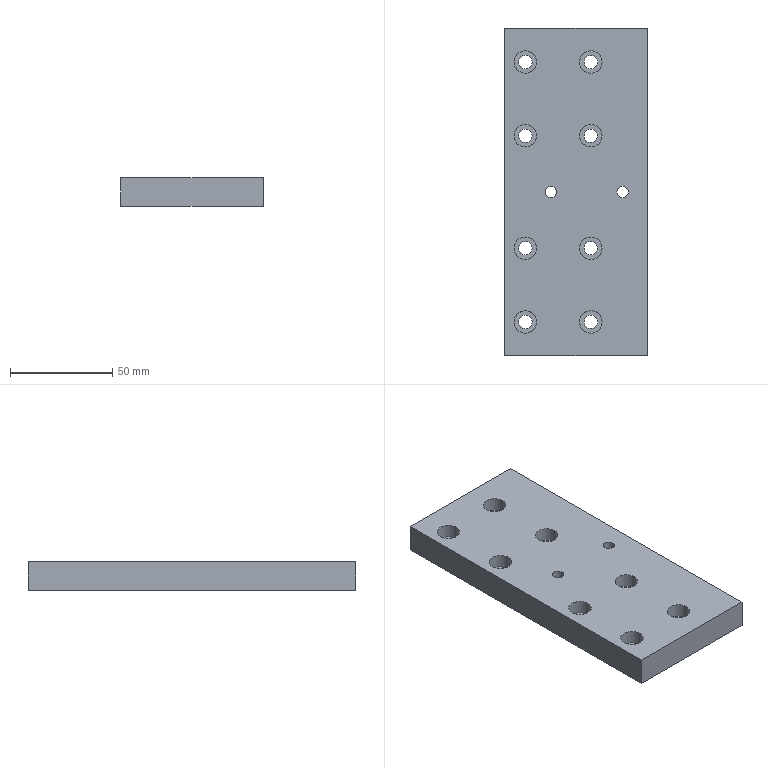Part | NX | 1 solid | 40 faces | box 69.5 x 160 x 14 mm | volume 146674 mm3 | cylinder 22 | plane 16 | cone 2 | commonest cylinder face diameters 6.6 x8 11 x8 5 x2 5.5 x2 10 x2
STEP:
#1=CARTESIAN_POINT('',(-34.75,80.,-7.));
#2=VERTEX_POINT('',#1);
#3=CARTESIAN_POINT('',(-34.75,-80.,-7.));
#4=VERTEX_POINT('',#3);
#5=CARTESIAN_POINT('',(-34.75,80.,-7.));
#6=DIRECTION('',(0.,-1.,0.));
#7=VECTOR('',#6,1000.);
#8=LINE('',#5,#7);
#9=EDGE_CURVE('',#2,#4,#8,.T.);
#10=ORIENTED_EDGE('',*,*,#9,.T.);
#11=CARTESIAN_POINT('',(-34.75,-80.,7.));
#12=VERTEX_POINT('',#11);
#13=CARTESIAN_POINT('',(-34.75,-80.,7.));
#14=DIRECTION('',(0.,0.,-1.));
#15=VECTOR('',#14,1000.);
#16=LINE('',#13,#15);
#17=EDGE_CURVE('',#12,#4,#16,.T.);
#18=ORIENTED_EDGE('',*,*,#17,.F.);
#19=CARTESIAN_POINT('',(-34.75,80.,7.));
#20=VERTEX_POINT('',#19);
#21=CARTESIAN_POINT('',(-34.75,80.,7.));
#22=DIRECTION('',(0.,-1.,0.));
#23=VECTOR('',#22,1000.);
#24=LINE('',#21,#23);
#25=EDGE_CURVE('',#20,#12,#24,.T.);
#26=ORIENTED_EDGE('',*,*,#25,.F.);
#27=CARTESIAN_POINT('',(-34.75,80.,7.));
#28=DIRECTION('',(0.,0.,-1.));
#29=VECTOR('',#28,1000.);
#30=LINE('',#27,#29);
#31=EDGE_CURVE('',#20,#2,#30,.T.);
#32=ORIENTED_EDGE('',*,*,#31,.T.);
#33=EDGE_LOOP('',(#10,#18,#26,#32));
#34=FACE_BOUND('',#33,.T.);
#35=CARTESIAN_POINT('',(-34.75,80.,7.));
#36=DIRECTION('',(1.,0.,0.));
#37=DIRECTION('',(0.,1.,0.));
#38=AXIS2_PLACEMENT_3D('',#35,#36,#37);
#39=PLANE('',#38);
#40=ADVANCED_FACE('',(#34),#39,.F.);
#41=CARTESIAN_POINT('',(34.75,-80.,-7.));
#42=VERTEX_POINT('',#41);
#43=CARTESIAN_POINT('',(34.75,-80.,-7.));
#44=DIRECTION('',(1.,0.,0.));
#45=VECTOR('',#44,1000.);
#46=LINE('',#43,#45);
#47=EDGE_CURVE('',#4,#42,#46,.T.);
#48=ORIENTED_EDGE('',*,*,#47,.T.);
#49=CARTESIAN_POINT('',(34.75,-80.,7.));
#50=VERTEX_POINT('',#49);
#51=CARTESIAN_POINT('',(34.75,-80.,7.));
#52=DIRECTION('',(0.,0.,-1.));
#53=VECTOR('',#52,1000.);
#54=LINE('',#51,#53);
#55=EDGE_CURVE('',#50,#42,#54,.T.);
#56=ORIENTED_EDGE('',*,*,#55,.F.);
#57=CARTESIAN_POINT('',(34.75,-80.,7.));
#58=DIRECTION('',(1.,0.,0.));
#59=VECTOR('',#58,1000.);
#60=LINE('',#57,#59);
#61=EDGE_CURVE('',#12,#50,#60,.T.);
#62=ORIENTED_EDGE('',*,*,#61,.F.);
#63=ORIENTED_EDGE('',*,*,#17,.T.);
#64=EDGE_LOOP('',(#48,#56,#62,#63));
#65=FACE_BOUND('',#64,.T.);
#66=CARTESIAN_POINT('',(34.75,-80.,7.));
#67=DIRECTION('',(0.,1.,0.));
#68=DIRECTION('',(0.,0.,1.));
#69=AXIS2_PLACEMENT_3D('',#66,#67,#68);
#70=PLANE('',#69);
#71=ADVANCED_FACE('',(#65),#70,.F.);
#72=CARTESIAN_POINT('',(34.75,32.5,-3.));
#73=VERTEX_POINT('',#72);
#74=CARTESIAN_POINT('',(34.75,32.5,-0.5));
#75=DIRECTION('',(1.,0.,0.));
#76=DIRECTION('',(0.,0.,-1.));
#77=AXIS2_PLACEMENT_3D('',#74,#75,#76);
#78=CIRCLE('',#77,2.5);
#79=EDGE_CURVE('',#73,#73,#78,.T.);
#80=ORIENTED_EDGE('',*,*,#79,.F.);
#81=EDGE_LOOP('',(#80));
#82=FACE_BOUND('',#81,.T.);
#83=CARTESIAN_POINT('',(34.75,-32.5,-3.));
#84=VERTEX_POINT('',#83);
#85=CARTESIAN_POINT('',(34.75,-32.5,-0.5));
#86=DIRECTION('',(1.,0.,0.));
#87=DIRECTION('',(0.,0.,-1.));
#88=AXIS2_PLACEMENT_3D('',#85,#86,#87);
#89=CIRCLE('',#88,2.5);
#90=EDGE_CURVE('',#84,#84,#89,.T.);
#91=ORIENTED_EDGE('',*,*,#90,.F.);
#92=EDGE_LOOP('',(#91));
#93=FACE_BOUND('',#92,.T.);
#94=CARTESIAN_POINT('',(34.75,80.,-7.));
#95=VERTEX_POINT('',#94);
#96=CARTESIAN_POINT('',(34.75,80.,-7.));
#97=DIRECTION('',(0.,1.,0.));
#98=VECTOR('',#97,1000.);
#99=LINE('',#96,#98);
#100=EDGE_CURVE('',#42,#95,#99,.T.);
#101=ORIENTED_EDGE('',*,*,#100,.T.);
#102=CARTESIAN_POINT('',(34.75,80.,7.));
#103=VERTEX_POINT('',#102);
#104=CARTESIAN_POINT('',(34.75,80.,7.));
#105=DIRECTION('',(0.,0.,-1.));
#106=VECTOR('',#105,1000.);
#107=LINE('',#104,#106);
#108=EDGE_CURVE('',#103,#95,#107,.T.);
#109=ORIENTED_EDGE('',*,*,#108,.F.);
#110=CARTESIAN_POINT('',(34.75,80.,7.));
#111=DIRECTION('',(0.,1.,0.));
#112=VECTOR('',#111,1000.);
#113=LINE('',#110,#112);
#114=EDGE_CURVE('',#50,#103,#113,.T.);
#115=ORIENTED_EDGE('',*,*,#114,.F.);
#116=ORIENTED_EDGE('',*,*,#55,.T.);
#117=EDGE_LOOP('',(#101,#109,#115,#116));
#118=FACE_BOUND('',#117,.T.);
#119=CARTESIAN_POINT('',(34.75,80.,7.));
#120=DIRECTION('',(-1.,0.,0.));
#121=DIRECTION('',(0.,-1.,0.));
#122=AXIS2_PLACEMENT_3D('',#119,#120,#121);
#123=PLANE('',#122);
#124=ADVANCED_FACE('',(#82,#93,#118),#123,.F.);
#125=CARTESIAN_POINT('',(34.75,80.,-7.));
#126=DIRECTION('',(-1.,0.,0.));
#127=VECTOR('',#126,1000.);
#128=LINE('',#125,#127);
#129=EDGE_CURVE('',#95,#2,#128,.T.);
#130=ORIENTED_EDGE('',*,*,#129,.T.);
#131=ORIENTED_EDGE('',*,*,#31,.F.);
#132=CARTESIAN_POINT('',(34.75,80.,7.));
#133=DIRECTION('',(-1.,0.,0.));
#134=VECTOR('',#133,1000.);
#135=LINE('',#132,#134);
#136=EDGE_CURVE('',#103,#20,#135,.T.);
#137=ORIENTED_EDGE('',*,*,#136,.F.);
#138=ORIENTED_EDGE('',*,*,#108,.T.);
#139=EDGE_LOOP('',(#130,#131,#137,#138));
#140=FACE_BOUND('',#139,.T.);
#141=CARTESIAN_POINT('',(34.75,80.,7.));
#142=DIRECTION('',(0.,-1.,0.));
#143=DIRECTION('',(0.,0.,-1.));
#144=AXIS2_PLACEMENT_3D('',#141,#142,#143);
#145=PLANE('',#144);
#146=ADVANCED_FACE('',(#140),#145,.F.);
#147=CARTESIAN_POINT('',(-15.,0.,7.));
#148=VERTEX_POINT('',#147);
#149=CARTESIAN_POINT('',(-12.25,0.,7.));
#150=DIRECTION('',(0.,0.,-1.));
#151=DIRECTION('',(-1.,0.,0.));
#152=AXIS2_PLACEMENT_3D('',#149,#150,#151);
#153=CIRCLE('',#152,2.75);
#154=EDGE_CURVE('',#148,#148,#153,.T.);
#155=ORIENTED_EDGE('',*,*,#154,.T.);
#156=EDGE_LOOP('',(#155));
#157=FACE_BOUND('',#156,.T.);
#158=CARTESIAN_POINT('',(20.,0.,7.));
#159=VERTEX_POINT('',#158);
#160=CARTESIAN_POINT('',(22.75,0.,7.));
#161=DIRECTION('',(0.,0.,-1.));
#162=DIRECTION('',(-1.,0.,0.));
#163=AXIS2_PLACEMENT_3D('',#160,#161,#162);
#164=CIRCLE('',#163,2.75);
#165=EDGE_CURVE('',#159,#159,#164,.T.);
#166=ORIENTED_EDGE('',*,*,#165,.T.);
#167=EDGE_LOOP('',(#166));
#168=FACE_BOUND('',#167,.T.);
#169=CARTESIAN_POINT('',(-19.25,27.5,7.));
#170=VERTEX_POINT('',#169);
#171=CARTESIAN_POINT('',(-24.75,27.5,7.));
#172=DIRECTION('',(0.,0.,1.));
#173=DIRECTION('',(1.,0.,0.));
#174=AXIS2_PLACEMENT_3D('',#171,#172,#173);
#175=CIRCLE('',#174,5.5);
#176=EDGE_CURVE('',#170,#170,#175,.T.);
#177=ORIENTED_EDGE('',*,*,#176,.F.);
#178=EDGE_LOOP('',(#177));
#179=FACE_BOUND('',#178,.T.);
#180=CARTESIAN_POINT('',(12.75,27.5,7.));
#181=VERTEX_POINT('',#180);
#182=CARTESIAN_POINT('',(7.25,27.5,7.));
#183=DIRECTION('',(0.,0.,1.));
#184=DIRECTION('',(1.,0.,0.));
#185=AXIS2_PLACEMENT_3D('',#182,#183,#184);
#186=CIRCLE('',#185,5.5);
#187=EDGE_CURVE('',#181,#181,#186,.T.);
#188=ORIENTED_EDGE('',*,*,#187,.F.);
#189=EDGE_LOOP('',(#188));
#190=FACE_BOUND('',#189,.T.);
#191=CARTESIAN_POINT('',(12.75,-27.5,7.));
#192=VERTEX_POINT('',#191);
#193=CARTESIAN_POINT('',(7.25,-27.5,7.));
#194=DIRECTION('',(0.,0.,1.));
#195=DIRECTION('',(1.,0.,0.));
#196=AXIS2_PLACEMENT_3D('',#193,#194,#195);
#197=CIRCLE('',#196,5.5);
#198=EDGE_CURVE('',#192,#192,#197,.T.);
#199=ORIENTED_EDGE('',*,*,#198,.F.);
#200=EDGE_LOOP('',(#199));
#201=FACE_BOUND('',#200,.T.);
#202=CARTESIAN_POINT('',(-19.25,-27.5,7.));
#203=VERTEX_POINT('',#202);
#204=CARTESIAN_POINT('',(-24.75,-27.5,7.));
#205=DIRECTION('',(0.,0.,1.));
#206=DIRECTION('',(1.,0.,0.));
#207=AXIS2_PLACEMENT_3D('',#204,#205,#206);
#208=CIRCLE('',#207,5.5);
#209=EDGE_CURVE('',#203,#203,#208,.T.);
#210=ORIENTED_EDGE('',*,*,#209,.F.);
#211=EDGE_LOOP('',(#210));
#212=FACE_BOUND('',#211,.T.);
#213=CARTESIAN_POINT('',(12.75,63.5,7.));
#214=VERTEX_POINT('',#213);
#215=CARTESIAN_POINT('',(7.25,63.5,7.));
#216=DIRECTION('',(0.,0.,1.));
#217=DIRECTION('',(1.,0.,0.));
#218=AXIS2_PLACEMENT_3D('',#215,#216,#217);
#219=CIRCLE('',#218,5.5);
#220=EDGE_CURVE('',#214,#214,#219,.T.);
#221=ORIENTED_EDGE('',*,*,#220,.F.);
#222=EDGE_LOOP('',(#221));
#223=FACE_BOUND('',#222,.T.);
#224=CARTESIAN_POINT('',(-19.25,63.5,7.));
#225=VERTEX_POINT('',#224);
#226=CARTESIAN_POINT('',(-24.75,63.5,7.));
#227=DIRECTION('',(0.,0.,1.));
#228=DIRECTION('',(1.,0.,0.));
#229=AXIS2_PLACEMENT_3D('',#226,#227,#228);
#230=CIRCLE('',#229,5.5);
#231=EDGE_CURVE('',#225,#225,#230,.T.);
#232=ORIENTED_EDGE('',*,*,#231,.F.);
#233=EDGE_LOOP('',(#232));
#234=FACE_BOUND('',#233,.T.);
#235=CARTESIAN_POINT('',(-19.25,-63.5,7.));
#236=VERTEX_POINT('',#235);
#237=CARTESIAN_POINT('',(-24.75,-63.5,7.));
#238=DIRECTION('',(0.,0.,1.));
#239=DIRECTION('',(1.,0.,0.));
#240=AXIS2_PLACEMENT_3D('',#237,#238,#239);
#241=CIRCLE('',#240,5.5);
#242=EDGE_CURVE('',#236,#236,#241,.T.);
#243=ORIENTED_EDGE('',*,*,#242,.F.);
#244=EDGE_LOOP('',(#243));
#245=FACE_BOUND('',#244,.T.);
#246=CARTESIAN_POINT('',(12.75,-63.5,7.));
#247=VERTEX_POINT('',#246);
#248=CARTESIAN_POINT('',(7.25,-63.5,7.));
#249=DIRECTION('',(0.,0.,1.));
#250=DIRECTION('',(1.,0.,0.));
#251=AXIS2_PLACEMENT_3D('',#248,#249,#250);
#252=CIRCLE('',#251,5.5);
#253=EDGE_CURVE('',#247,#247,#252,.T.);
#254=ORIENTED_EDGE('',*,*,#253,.F.);
#255=EDGE_LOOP('',(#254));
#256=FACE_BOUND('',#255,.T.);
#257=ORIENTED_EDGE('',*,*,#25,.T.);
#258=ORIENTED_EDGE('',*,*,#61,.T.);
#259=ORIENTED_EDGE('',*,*,#114,.T.);
#260=ORIENTED_EDGE('',*,*,#136,.T.);
#261=EDGE_LOOP('',(#257,#258,#259,#260));
#262=FACE_BOUND('',#261,.T.);
#263=CARTESIAN_POINT('',(0.,0.,7.));
#264=DIRECTION('',(0.,0.,-1.));
#265=DIRECTION('',(-1.,0.,0.));
#266=AXIS2_PLACEMENT_3D('',#263,#264,#265);
#267=PLANE('',#266);
#268=ADVANCED_FACE('',(#157,#168,#179,#190,#201,#212,#223,#234,#245,#256,#262),#267,.F.);
#269=CARTESIAN_POINT('',(-17.25,0.,-7.));
#270=VERTEX_POINT('',#269);
#271=CARTESIAN_POINT('',(-12.25,0.,-7.));
#272=DIRECTION('',(0.,0.,-1.));
#273=DIRECTION('',(-1.,0.,0.));
#274=AXIS2_PLACEMENT_3D('',#271,#272,#273);
#275=CIRCLE('',#274,5.);
#276=EDGE_CURVE('',#270,#270,#275,.T.);
#277=ORIENTED_EDGE('',*,*,#276,.F.);
#278=EDGE_LOOP('',(#277));
#279=FACE_BOUND('',#278,.T.);
#280=CARTESIAN_POINT('',(17.75,0.,-7.));
#281=VERTEX_POINT('',#280);
#282=CARTESIAN_POINT('',(22.75,0.,-7.));
#283=DIRECTION('',(0.,0.,-1.));
#284=DIRECTION('',(-1.,0.,0.));
#285=AXIS2_PLACEMENT_3D('',#282,#283,#284);
#286=CIRCLE('',#285,5.);
#287=EDGE_CURVE('',#281,#281,#286,.T.);
#288=ORIENTED_EDGE('',*,*,#287,.F.);
#289=EDGE_LOOP('',(#288));
#290=FACE_BOUND('',#289,.T.);
#291=CARTESIAN_POINT('',(-21.45,27.5,-7.));
#292=VERTEX_POINT('',#291);
#293=CARTESIAN_POINT('',(-24.75,27.5,-7.));
#294=DIRECTION('',(0.,0.,1.));
#295=DIRECTION('',(1.,0.,0.));
#296=AXIS2_PLACEMENT_3D('',#293,#294,#295);
#297=CIRCLE('',#296,3.3);
#298=EDGE_CURVE('',#292,#292,#297,.T.);
#299=ORIENTED_EDGE('',*,*,#298,.T.);
#300=EDGE_LOOP('',(#299));
#301=FACE_BOUND('',#300,.T.);
#302=CARTESIAN_POINT('',(10.55,27.5,-7.));
#303=VERTEX_POINT('',#302);
#304=CARTESIAN_POINT('',(7.25,27.5,-7.));
#305=DIRECTION('',(0.,0.,1.));
#306=DIRECTION('',(1.,0.,0.));
#307=AXIS2_PLACEMENT_3D('',#304,#305,#306);
#308=CIRCLE('',#307,3.3);
#309=EDGE_CURVE('',#303,#303,#308,.T.);
#310=ORIENTED_EDGE('',*,*,#309,.T.);
#311=EDGE_LOOP('',(#310));
#312=FACE_BOUND('',#311,.T.);
#313=CARTESIAN_POINT('',(10.55,-27.5,-7.));
#314=VERTEX_POINT('',#313);
#315=CARTESIAN_POINT('',(7.25,-27.5,-7.));
#316=DIRECTION('',(0.,0.,1.));
#317=DIRECTION('',(1.,0.,0.));
#318=AXIS2_PLACEMENT_3D('',#315,#316,#317);
#319=CIRCLE('',#318,3.3);
#320=EDGE_CURVE('',#314,#314,#319,.T.);
#321=ORIENTED_EDGE('',*,*,#320,.T.);
#322=EDGE_LOOP('',(#321));
#323=FACE_BOUND('',#322,.T.);
#324=CARTESIAN_POINT('',(-21.45,-27.5,-7.));
#325=VERTEX_POINT('',#324);
#326=CARTESIAN_POINT('',(-24.75,-27.5,-7.));
#327=DIRECTION('',(0.,0.,1.));
#328=DIRECTION('',(1.,0.,0.));
#329=AXIS2_PLACEMENT_3D('',#326,#327,#328);
#330=CIRCLE('',#329,3.3);
#331=EDGE_CURVE('',#325,#325,#330,.T.);
#332=ORIENTED_EDGE('',*,*,#331,.T.);
#333=EDGE_LOOP('',(#332));
#334=FACE_BOUND('',#333,.T.);
#335=CARTESIAN_POINT('',(10.55,63.5,-7.));
#336=VERTEX_POINT('',#335);
#337=CARTESIAN_POINT('',(7.25,63.5,-7.));
#338=DIRECTION('',(0.,0.,1.));
#339=DIRECTION('',(1.,0.,0.));
#340=AXIS2_PLACEMENT_3D('',#337,#338,#339);
#341=CIRCLE('',#340,3.3);
#342=EDGE_CURVE('',#336,#336,#341,.T.);
#343=ORIENTED_EDGE('',*,*,#342,.T.);
#344=EDGE_LOOP('',(#343));
#345=FACE_BOUND('',#344,.T.);
#346=CARTESIAN_POINT('',(-21.45,63.5,-7.));
#347=VERTEX_POINT('',#346);
#348=CARTESIAN_POINT('',(-24.75,63.5,-7.));
#349=DIRECTION('',(0.,0.,1.));
#350=DIRECTION('',(1.,0.,0.));
#351=AXIS2_PLACEMENT_3D('',#348,#349,#350);
#352=CIRCLE('',#351,3.3);
#353=EDGE_CURVE('',#347,#347,#352,.T.);
#354=ORIENTED_EDGE('',*,*,#353,.T.);
#355=EDGE_LOOP('',(#354));
#356=FACE_BOUND('',#355,.T.);
#357=CARTESIAN_POINT('',(-21.45,-63.5,-7.));
#358=VERTEX_POINT('',#357);
#359=CARTESIAN_POINT('',(-24.75,-63.5,-7.));
#360=DIRECTION('',(0.,0.,1.));
#361=DIRECTION('',(1.,0.,0.));
#362=AXIS2_PLACEMENT_3D('',#359,#360,#361);
#363=CIRCLE('',#362,3.3);
#364=EDGE_CURVE('',#358,#358,#363,.T.);
#365=ORIENTED_EDGE('',*,*,#364,.T.);
#366=EDGE_LOOP('',(#365));
#367=FACE_BOUND('',#366,.T.);
#368=CARTESIAN_POINT('',(10.55,-63.5,-7.));
#369=VERTEX_POINT('',#368);
#370=CARTESIAN_POINT('',(7.25,-63.5,-7.));
#371=DIRECTION('',(0.,0.,1.));
#372=DIRECTION('',(1.,0.,0.));
#373=AXIS2_PLACEMENT_3D('',#370,#371,#372);
#374=CIRCLE('',#373,3.3);
#375=EDGE_CURVE('',#369,#369,#374,.T.);
#376=ORIENTED_EDGE('',*,*,#375,.T.);
#377=EDGE_LOOP('',(#376));
#378=FACE_BOUND('',#377,.T.);
#379=ORIENTED_EDGE('',*,*,#9,.F.);
#380=ORIENTED_EDGE('',*,*,#129,.F.);
#381=ORIENTED_EDGE('',*,*,#100,.F.);
#382=ORIENTED_EDGE('',*,*,#47,.F.);
#383=EDGE_LOOP('',(#379,#380,#381,#382));
#384=FACE_BOUND('',#383,.T.);
#385=CARTESIAN_POINT('',(0.,0.,-7.));
#386=DIRECTION('',(0.,0.,-1.));
#387=DIRECTION('',(-1.,0.,0.));
#388=AXIS2_PLACEMENT_3D('',#385,#386,#387);
#389=PLANE('',#388);
#390=ADVANCED_FACE('',(#279,#290,#301,#312,#323,#334,#345,#356,#367,#378,#384),#389,.T.);
#391=ORIENTED_EDGE('',*,*,#375,.F.);
#392=EDGE_LOOP('',(#391));
#393=FACE_BOUND('',#392,.T.);
#394=CARTESIAN_POINT('',(10.55,-63.5,0.2));
#395=VERTEX_POINT('',#394);
#396=CARTESIAN_POINT('',(7.25,-63.5,0.2));
#397=DIRECTION('',(0.,0.,1.));
#398=DIRECTION('',(1.,0.,0.));
#399=AXIS2_PLACEMENT_3D('',#396,#397,#398);
#400=CIRCLE('',#399,3.3);
#401=EDGE_CURVE('',#395,#395,#400,.T.);
#402=ORIENTED_EDGE('',*,*,#401,.T.);
#403=EDGE_LOOP('',(#402));
#404=FACE_BOUND('',#403,.T.);
#405=CARTESIAN_POINT('',(7.25,-63.5,7.));
#406=DIRECTION('',(0.,0.,1.));
#407=DIRECTION('',(1.,0.,0.));
#408=AXIS2_PLACEMENT_3D('',#405,#406,#407);
#409=CYLINDRICAL_SURFACE('',#408,3.3);
#410=ADVANCED_FACE('',(#393,#404),#409,.F.);
#411=ORIENTED_EDGE('',*,*,#401,.F.);
#412=EDGE_LOOP('',(#411));
#413=FACE_BOUND('',#412,.T.);
#414=CARTESIAN_POINT('',(12.75,-63.5,0.2));
#415=VERTEX_POINT('',#414);
#416=CARTESIAN_POINT('',(7.25,-63.5,0.2));
#417=DIRECTION('',(0.,0.,1.));
#418=DIRECTION('',(1.,0.,0.));
#419=AXIS2_PLACEMENT_3D('',#416,#417,#418);
#420=CIRCLE('',#419,5.5);
#421=EDGE_CURVE('',#415,#415,#420,.T.);
#422=ORIENTED_EDGE('',*,*,#421,.T.);
#423=EDGE_LOOP('',(#422));
#424=FACE_BOUND('',#423,.T.);
#425=CARTESIAN_POINT('',(10.55,-63.5,0.2));
#426=DIRECTION('',(0.,0.,-1.));
#427=DIRECTION('',(-1.,0.,0.));
#428=AXIS2_PLACEMENT_3D('',#425,#426,#427);
#429=PLANE('',#428);
#430=ADVANCED_FACE('',(#413,#424),#429,.F.);
#431=ORIENTED_EDGE('',*,*,#421,.F.);
#432=EDGE_LOOP('',(#431));
#433=FACE_BOUND('',#432,.T.);
#434=ORIENTED_EDGE('',*,*,#253,.T.);
#435=EDGE_LOOP('',(#434));
#436=FACE_BOUND('',#435,.T.);
#437=CARTESIAN_POINT('',(7.25,-63.5,7.));
#438=DIRECTION('',(0.,0.,1.));
#439=DIRECTION('',(1.,0.,0.));
#440=AXIS2_PLACEMENT_3D('',#437,#438,#439);
#441=CYLINDRICAL_SURFACE('',#440,5.5);
#442=ADVANCED_FACE('',(#433,#436),#441,.F.);
#443=ORIENTED_EDGE('',*,*,#364,.F.);
#444=EDGE_LOOP('',(#443));
#445=FACE_BOUND('',#444,.T.);
#446=CARTESIAN_POINT('',(-21.45,-63.5,0.2));
#447=VERTEX_POINT('',#446);
#448=CARTESIAN_POINT('',(-24.75,-63.5,0.2));
#449=DIRECTION('',(0.,0.,1.));
#450=DIRECTION('',(1.,0.,0.));
#451=AXIS2_PLACEMENT_3D('',#448,#449,#450);
#452=CIRCLE('',#451,3.3);
#453=EDGE_CURVE('',#447,#447,#452,.T.);
#454=ORIENTED_EDGE('',*,*,#453,.T.);
#455=EDGE_LOOP('',(#454));
#456=FACE_BOUND('',#455,.T.);
#457=CARTESIAN_POINT('',(-24.75,-63.5,7.));
#458=DIRECTION('',(0.,0.,1.));
#459=DIRECTION('',(1.,0.,0.));
#460=AXIS2_PLACEMENT_3D('',#457,#458,#459);
#461=CYLINDRICAL_SURFACE('',#460,3.3);
#462=ADVANCED_FACE('',(#445,#456),#461,.F.);
#463=ORIENTED_EDGE('',*,*,#453,.F.);
#464=EDGE_LOOP('',(#463));
#465=FACE_BOUND('',#464,.T.);
#466=CARTESIAN_POINT('',(-19.25,-63.5,0.2));
#467=VERTEX_POINT('',#466);
#468=CARTESIAN_POINT('',(-24.75,-63.5,0.2));
#469=DIRECTION('',(0.,0.,1.));
#470=DIRECTION('',(1.,0.,0.));
#471=AXIS2_PLACEMENT_3D('',#468,#469,#470);
#472=CIRCLE('',#471,5.5);
#473=EDGE_CURVE('',#467,#467,#472,.T.);
#474=ORIENTED_EDGE('',*,*,#473,.T.);
#475=EDGE_LOOP('',(#474));
#476=FACE_BOUND('',#475,.T.);
#477=CARTESIAN_POINT('',(-21.45,-63.5,0.2));
#478=DIRECTION('',(0.,0.,-1.));
#479=DIRECTION('',(-1.,0.,0.));
#480=AXIS2_PLACEMENT_3D('',#477,#478,#479);
#481=PLANE('',#480);
#482=ADVANCED_FACE('',(#465,#476),#481,.F.);
#483=ORIENTED_EDGE('',*,*,#473,.F.);
#484=EDGE_LOOP('',(#483));
#485=FACE_BOUND('',#484,.T.);
#486=ORIENTED_EDGE('',*,*,#242,.T.);
#487=EDGE_LOOP('',(#486));
#488=FACE_BOUND('',#487,.T.);
#489=CARTESIAN_POINT('',(-24.75,-63.5,7.));
#490=DIRECTION('',(0.,0.,1.));
#491=DIRECTION('',(1.,0.,0.));
#492=AXIS2_PLACEMENT_3D('',#489,#490,#491);
#493=CYLINDRICAL_SURFACE('',#492,5.5);
#494=ADVANCED_FACE('',(#485,#488),#493,.F.);
#495=ORIENTED_EDGE('',*,*,#353,.F.);
#496=EDGE_LOOP('',(#495));
#497=FACE_BOUND('',#496,.T.);
#498=CARTESIAN_POINT('',(-21.45,63.5,0.2));
#499=VERTEX_POINT('',#498);
#500=CARTESIAN_POINT('',(-24.75,63.5,0.2));
#501=DIRECTION('',(0.,0.,1.));
#502=DIRECTION('',(1.,0.,0.));
#503=AXIS2_PLACEMENT_3D('',#500,#501,#502);
#504=CIRCLE('',#503,3.3);
#505=EDGE_CURVE('',#499,#499,#504,.T.);
#506=ORIENTED_EDGE('',*,*,#505,.T.);
#507=EDGE_LOOP('',(#506));
#508=FACE_BOUND('',#507,.T.);
#509=CARTESIAN_POINT('',(-24.75,63.5,7.));
#510=DIRECTION('',(0.,0.,1.));
#511=DIRECTION('',(1.,0.,0.));
#512=AXIS2_PLACEMENT_3D('',#509,#510,#511);
#513=CYLINDRICAL_SURFACE('',#512,3.3);
#514=ADVANCED_FACE('',(#497,#508),#513,.F.);
#515=ORIENTED_EDGE('',*,*,#505,.F.);
#516=EDGE_LOOP('',(#515));
#517=FACE_BOUND('',#516,.T.);
#518=CARTESIAN_POINT('',(-19.25,63.5,0.2));
#519=VERTEX_POINT('',#518);
#520=CARTESIAN_POINT('',(-24.75,63.5,0.2));
#521=DIRECTION('',(0.,0.,1.));
#522=DIRECTION('',(1.,0.,0.));
#523=AXIS2_PLACEMENT_3D('',#520,#521,#522);
#524=CIRCLE('',#523,5.5);
#525=EDGE_CURVE('',#519,#519,#524,.T.);
#526=ORIENTED_EDGE('',*,*,#525,.T.);
#527=EDGE_LOOP('',(#526));
#528=FACE_BOUND('',#527,.T.);
#529=CARTESIAN_POINT('',(-21.45,63.5,0.2));
#530=DIRECTION('',(0.,0.,-1.));
#531=DIRECTION('',(-1.,0.,0.));
#532=AXIS2_PLACEMENT_3D('',#529,#530,#531);
#533=PLANE('',#532);
#534=ADVANCED_FACE('',(#517,#528),#533,.F.);
#535=ORIENTED_EDGE('',*,*,#525,.F.);
#536=EDGE_LOOP('',(#535));
#537=FACE_BOUND('',#536,.T.);
#538=ORIENTED_EDGE('',*,*,#231,.T.);
#539=EDGE_LOOP('',(#538));
#540=FACE_BOUND('',#539,.T.);
#541=CARTESIAN_POINT('',(-24.75,63.5,7.));
#542=DIRECTION('',(0.,0.,1.));
#543=DIRECTION('',(1.,0.,0.));
#544=AXIS2_PLACEMENT_3D('',#541,#542,#543);
#545=CYLINDRICAL_SURFACE('',#544,5.5);
#546=ADVANCED_FACE('',(#537,#540),#545,.F.);
#547=ORIENTED_EDGE('',*,*,#342,.F.);
#548=EDGE_LOOP('',(#547));
#549=FACE_BOUND('',#548,.T.);
#550=CARTESIAN_POINT('',(10.55,63.5,0.2));
#551=VERTEX_POINT('',#550);
#552=CARTESIAN_POINT('',(7.25,63.5,0.2));
#553=DIRECTION('',(0.,0.,1.));
#554=DIRECTION('',(1.,0.,0.));
#555=AXIS2_PLACEMENT_3D('',#552,#553,#554);
#556=CIRCLE('',#555,3.3);
#557=EDGE_CURVE('',#551,#551,#556,.T.);
#558=ORIENTED_EDGE('',*,*,#557,.T.);
#559=EDGE_LOOP('',(#558));
#560=FACE_BOUND('',#559,.T.);
#561=CARTESIAN_POINT('',(7.25,63.5,7.));
#562=DIRECTION('',(0.,0.,1.));
#563=DIRECTION('',(1.,0.,0.));
#564=AXIS2_PLACEMENT_3D('',#561,#562,#563);
#565=CYLINDRICAL_SURFACE('',#564,3.3);
#566=ADVANCED_FACE('',(#549,#560),#565,.F.);
#567=ORIENTED_EDGE('',*,*,#557,.F.);
#568=EDGE_LOOP('',(#567));
#569=FACE_BOUND('',#568,.T.);
#570=CARTESIAN_POINT('',(12.75,63.5,0.2));
#571=VERTEX_POINT('',#570);
#572=CARTESIAN_POINT('',(7.25,63.5,0.2));
#573=DIRECTION('',(0.,0.,1.));
#574=DIRECTION('',(1.,0.,0.));
#575=AXIS2_PLACEMENT_3D('',#572,#573,#574);
#576=CIRCLE('',#575,5.5);
#577=EDGE_CURVE('',#571,#571,#576,.T.);
#578=ORIENTED_EDGE('',*,*,#577,.T.);
#579=EDGE_LOOP('',(#578));
#580=FACE_BOUND('',#579,.T.);
#581=CARTESIAN_POINT('',(10.55,63.5,0.2));
#582=DIRECTION('',(0.,0.,-1.));
#583=DIRECTION('',(-1.,0.,0.));
#584=AXIS2_PLACEMENT_3D('',#581,#582,#583);
#585=PLANE('',#584);
#586=ADVANCED_FACE('',(#569,#580),#585,.F.);
#587=ORIENTED_EDGE('',*,*,#577,.F.);
#588=EDGE_LOOP('',(#587));
#589=FACE_BOUND('',#588,.T.);
#590=ORIENTED_EDGE('',*,*,#220,.T.);
#591=EDGE_LOOP('',(#590));
#592=FACE_BOUND('',#591,.T.);
#593=CARTESIAN_POINT('',(7.25,63.5,7.));
#594=DIRECTION('',(0.,0.,1.));
#595=DIRECTION('',(1.,0.,0.));
#596=AXIS2_PLACEMENT_3D('',#593,#594,#595);
#597=CYLINDRICAL_SURFACE('',#596,5.5);
#598=ADVANCED_FACE('',(#589,#592),#597,.F.);
#599=ORIENTED_EDGE('',*,*,#331,.F.);
#600=EDGE_LOOP('',(#599));
#601=FACE_BOUND('',#600,.T.);
#602=CARTESIAN_POINT('',(-21.45,-27.5,0.2));
#603=VERTEX_POINT('',#602);
#604=CARTESIAN_POINT('',(-24.75,-27.5,0.2));
#605=DIRECTION('',(0.,0.,1.));
#606=DIRECTION('',(1.,0.,0.));
#607=AXIS2_PLACEMENT_3D('',#604,#605,#606);
#608=CIRCLE('',#607,3.3);
#609=EDGE_CURVE('',#603,#603,#608,.T.);
#610=ORIENTED_EDGE('',*,*,#609,.T.);
#611=EDGE_LOOP('',(#610));
#612=FACE_BOUND('',#611,.T.);
#613=CARTESIAN_POINT('',(-24.75,-27.5,7.));
#614=DIRECTION('',(0.,0.,1.));
#615=DIRECTION('',(1.,0.,0.));
#616=AXIS2_PLACEMENT_3D('',#613,#614,#615);
#617=CYLINDRICAL_SURFACE('',#616,3.3);
#618=ADVANCED_FACE('',(#601,#612),#617,.F.);
#619=ORIENTED_EDGE('',*,*,#609,.F.);
#620=EDGE_LOOP('',(#619));
#621=FACE_BOUND('',#620,.T.);
#622=CARTESIAN_POINT('',(-19.25,-27.5,0.2));
#623=VERTEX_POINT('',#622);
#624=CARTESIAN_POINT('',(-24.75,-27.5,0.2));
#625=DIRECTION('',(0.,0.,1.));
#626=DIRECTION('',(1.,0.,0.));
#627=AXIS2_PLACEMENT_3D('',#624,#625,#626);
#628=CIRCLE('',#627,5.5);
#629=EDGE_CURVE('',#623,#623,#628,.T.);
#630=ORIENTED_EDGE('',*,*,#629,.T.);
#631=EDGE_LOOP('',(#630));
#632=FACE_BOUND('',#631,.T.);
#633=CARTESIAN_POINT('',(-21.45,-27.5,0.2));
#634=DIRECTION('',(0.,0.,-1.));
#635=DIRECTION('',(-1.,0.,0.));
#636=AXIS2_PLACEMENT_3D('',#633,#634,#635);
#637=PLANE('',#636);
#638=ADVANCED_FACE('',(#621,#632),#637,.F.);
#639=ORIENTED_EDGE('',*,*,#629,.F.);
#640=EDGE_LOOP('',(#639));
#641=FACE_BOUND('',#640,.T.);
#642=ORIENTED_EDGE('',*,*,#209,.T.);
#643=EDGE_LOOP('',(#642));
#644=FACE_BOUND('',#643,.T.);
#645=CARTESIAN_POINT('',(-24.75,-27.5,7.));
#646=DIRECTION('',(0.,0.,1.));
#647=DIRECTION('',(1.,0.,0.));
#648=AXIS2_PLACEMENT_3D('',#645,#646,#647);
#649=CYLINDRICAL_SURFACE('',#648,5.5);
#650=ADVANCED_FACE('',(#641,#644),#649,.F.);
#651=ORIENTED_EDGE('',*,*,#320,.F.);
#652=EDGE_LOOP('',(#651));
#653=FACE_BOUND('',#652,.T.);
#654=CARTESIAN_POINT('',(10.55,-27.5,0.2));
#655=VERTEX_POINT('',#654);
#656=CARTESIAN_POINT('',(7.25,-27.5,0.2));
#657=DIRECTION('',(0.,0.,1.));
#658=DIRECTION('',(1.,0.,0.));
#659=AXIS2_PLACEMENT_3D('',#656,#657,#658);
#660=CIRCLE('',#659,3.3);
#661=EDGE_CURVE('',#655,#655,#660,.T.);
#662=ORIENTED_EDGE('',*,*,#661,.T.);
#663=EDGE_LOOP('',(#662));
#664=FACE_BOUND('',#663,.T.);
#665=CARTESIAN_POINT('',(7.25,-27.5,7.));
#666=DIRECTION('',(0.,0.,1.));
#667=DIRECTION('',(1.,0.,0.));
#668=AXIS2_PLACEMENT_3D('',#665,#666,#667);
#669=CYLINDRICAL_SURFACE('',#668,3.3);
#670=ADVANCED_FACE('',(#653,#664),#669,.F.);
#671=ORIENTED_EDGE('',*,*,#661,.F.);
#672=EDGE_LOOP('',(#671));
#673=FACE_BOUND('',#672,.T.);
#674=CARTESIAN_POINT('',(12.75,-27.5,0.2));
#675=VERTEX_POINT('',#674);
#676=CARTESIAN_POINT('',(7.25,-27.5,0.2));
#677=DIRECTION('',(0.,0.,1.));
#678=DIRECTION('',(1.,0.,0.));
#679=AXIS2_PLACEMENT_3D('',#676,#677,#678);
#680=CIRCLE('',#679,5.5);
#681=EDGE_CURVE('',#675,#675,#680,.T.);
#682=ORIENTED_EDGE('',*,*,#681,.T.);
#683=EDGE_LOOP('',(#682));
#684=FACE_BOUND('',#683,.T.);
#685=CARTESIAN_POINT('',(10.55,-27.5,0.2));
#686=DIRECTION('',(0.,0.,-1.));
#687=DIRECTION('',(-1.,0.,0.));
#688=AXIS2_PLACEMENT_3D('',#685,#686,#687);
#689=PLANE('',#688);
#690=ADVANCED_FACE('',(#673,#684),#689,.F.);
#691=ORIENTED_EDGE('',*,*,#681,.F.);
#692=EDGE_LOOP('',(#691));
#693=FACE_BOUND('',#692,.T.);
#694=ORIENTED_EDGE('',*,*,#198,.T.);
#695=EDGE_LOOP('',(#694));
#696=FACE_BOUND('',#695,.T.);
#697=CARTESIAN_POINT('',(7.25,-27.5,7.));
#698=DIRECTION('',(0.,0.,1.));
#699=DIRECTION('',(1.,0.,0.));
#700=AXIS2_PLACEMENT_3D('',#697,#698,#699);
#701=CYLINDRICAL_SURFACE('',#700,5.5);
#702=ADVANCED_FACE('',(#693,#696),#701,.F.);
#703=ORIENTED_EDGE('',*,*,#309,.F.);
#704=EDGE_LOOP('',(#703));
#705=FACE_BOUND('',#704,.T.);
#706=CARTESIAN_POINT('',(10.55,27.5,0.2));
#707=VERTEX_POINT('',#706);
#708=CARTESIAN_POINT('',(7.25,27.5,0.2));
#709=DIRECTION('',(0.,0.,1.));
#710=DIRECTION('',(1.,0.,0.));
#711=AXIS2_PLACEMENT_3D('',#708,#709,#710);
#712=CIRCLE('',#711,3.3);
#713=EDGE_CURVE('',#707,#707,#712,.T.);
#714=ORIENTED_EDGE('',*,*,#713,.T.);
#715=EDGE_LOOP('',(#714));
#716=FACE_BOUND('',#715,.T.);
#717=CARTESIAN_POINT('',(7.25,27.5,7.));
#718=DIRECTION('',(0.,0.,1.));
#719=DIRECTION('',(1.,0.,0.));
#720=AXIS2_PLACEMENT_3D('',#717,#718,#719);
#721=CYLINDRICAL_SURFACE('',#720,3.3);
#722=ADVANCED_FACE('',(#705,#716),#721,.F.);
#723=ORIENTED_EDGE('',*,*,#713,.F.);
#724=EDGE_LOOP('',(#723));
#725=FACE_BOUND('',#724,.T.);
#726=CARTESIAN_POINT('',(12.75,27.5,0.2));
#727=VERTEX_POINT('',#726);
#728=CARTESIAN_POINT('',(7.25,27.5,0.2));
#729=DIRECTION('',(0.,0.,1.));
#730=DIRECTION('',(1.,0.,0.));
#731=AXIS2_PLACEMENT_3D('',#728,#729,#730);
#732=CIRCLE('',#731,5.5);
#733=EDGE_CURVE('',#727,#727,#732,.T.);
#734=ORIENTED_EDGE('',*,*,#733,.T.);
#735=EDGE_LOOP('',(#734));
#736=FACE_BOUND('',#735,.T.);
#737=CARTESIAN_POINT('',(10.55,27.5,0.2));
#738=DIRECTION('',(0.,0.,-1.));
#739=DIRECTION('',(-1.,0.,0.));
#740=AXIS2_PLACEMENT_3D('',#737,#738,#739);
#741=PLANE('',#740);
#742=ADVANCED_FACE('',(#725,#736),#741,.F.);
#743=ORIENTED_EDGE('',*,*,#733,.F.);
#744=EDGE_LOOP('',(#743));
#745=FACE_BOUND('',#744,.T.);
#746=ORIENTED_EDGE('',*,*,#187,.T.);
#747=EDGE_LOOP('',(#746));
#748=FACE_BOUND('',#747,.T.);
#749=CARTESIAN_POINT('',(7.25,27.5,7.));
#750=DIRECTION('',(0.,0.,1.));
#751=DIRECTION('',(1.,0.,0.));
#752=AXIS2_PLACEMENT_3D('',#749,#750,#751);
#753=CYLINDRICAL_SURFACE('',#752,5.5);
#754=ADVANCED_FACE('',(#745,#748),#753,.F.);
#755=ORIENTED_EDGE('',*,*,#298,.F.);
#756=EDGE_LOOP('',(#755));
#757=FACE_BOUND('',#756,.T.);
#758=CARTESIAN_POINT('',(-21.45,27.5,0.2));
#759=VERTEX_POINT('',#758);
#760=CARTESIAN_POINT('',(-24.75,27.5,0.2));
#761=DIRECTION('',(0.,0.,1.));
#762=DIRECTION('',(1.,0.,0.));
#763=AXIS2_PLACEMENT_3D('',#760,#761,#762);
#764=CIRCLE('',#763,3.3);
#765=EDGE_CURVE('',#759,#759,#764,.T.);
#766=ORIENTED_EDGE('',*,*,#765,.T.);
#767=EDGE_LOOP('',(#766));
#768=FACE_BOUND('',#767,.T.);
#769=CARTESIAN_POINT('',(-24.75,27.5,7.));
#770=DIRECTION('',(0.,0.,1.));
#771=DIRECTION('',(1.,0.,0.));
#772=AXIS2_PLACEMENT_3D('',#769,#770,#771);
#773=CYLINDRICAL_SURFACE('',#772,3.3);
#774=ADVANCED_FACE('',(#757,#768),#773,.F.);
#775=ORIENTED_EDGE('',*,*,#765,.F.);
#776=EDGE_LOOP('',(#775));
#777=FACE_BOUND('',#776,.T.);
#778=CARTESIAN_POINT('',(-19.25,27.5,0.2));
#779=VERTEX_POINT('',#778);
#780=CARTESIAN_POINT('',(-24.75,27.5,0.2));
#781=DIRECTION('',(0.,0.,1.));
#782=DIRECTION('',(1.,0.,0.));
#783=AXIS2_PLACEMENT_3D('',#780,#781,#782);
#784=CIRCLE('',#783,5.5);
#785=EDGE_CURVE('',#779,#779,#784,.T.);
#786=ORIENTED_EDGE('',*,*,#785,.T.);
#787=EDGE_LOOP('',(#786));
#788=FACE_BOUND('',#787,.T.);
#789=CARTESIAN_POINT('',(-21.45,27.5,0.2));
#790=DIRECTION('',(0.,0.,-1.));
#791=DIRECTION('',(-1.,0.,0.));
#792=AXIS2_PLACEMENT_3D('',#789,#790,#791);
#793=PLANE('',#792);
#794=ADVANCED_FACE('',(#777,#788),#793,.F.);
#795=ORIENTED_EDGE('',*,*,#785,.F.);
#796=EDGE_LOOP('',(#795));
#797=FACE_BOUND('',#796,.T.);
#798=ORIENTED_EDGE('',*,*,#176,.T.);
#799=EDGE_LOOP('',(#798));
#800=FACE_BOUND('',#799,.T.);
#801=CARTESIAN_POINT('',(-24.75,27.5,7.));
#802=DIRECTION('',(0.,0.,1.));
#803=DIRECTION('',(1.,0.,0.));
#804=AXIS2_PLACEMENT_3D('',#801,#802,#803);
#805=CYLINDRICAL_SURFACE('',#804,5.5);
#806=ADVANCED_FACE('',(#797,#800),#805,.F.);
#807=CARTESIAN_POINT('',(18.248,-32.5,-0.5));
#808=VERTEX_POINT('',#807);
#809=VERTEX_LOOP('',#808);
#810=FACE_BOUND('',#809,.T.);
#811=CARTESIAN_POINT('',(19.75,-32.5,-3.));
#812=VERTEX_POINT('',#811);
#813=CARTESIAN_POINT('',(19.75,-32.5,-0.5));
#814=DIRECTION('',(1.,0.,0.));
#815=DIRECTION('',(0.,0.,-1.));
#816=AXIS2_PLACEMENT_3D('',#813,#814,#815);
#817=CIRCLE('',#816,2.5);
#818=EDGE_CURVE('',#812,#812,#817,.T.);
#819=ORIENTED_EDGE('',*,*,#818,.T.);
#820=EDGE_LOOP('',(#819));
#821=FACE_BOUND('',#820,.T.);
#822=CARTESIAN_POINT('',(19.75,-32.5,-0.5));
#823=DIRECTION('',(1.,0.,0.));
#824=DIRECTION('',(0.,0.,-1.));
#825=AXIS2_PLACEMENT_3D('',#822,#823,#824);
#826=CONICAL_SURFACE('',#825,2.5,1.03);
#827=ADVANCED_FACE('',(#810,#821),#826,.F.);
#828=ORIENTED_EDGE('',*,*,#818,.F.);
#829=EDGE_LOOP('',(#828));
#830=FACE_BOUND('',#829,.T.);
#831=ORIENTED_EDGE('',*,*,#90,.T.);
#832=EDGE_LOOP('',(#831));
#833=FACE_BOUND('',#832,.T.);
#834=CARTESIAN_POINT('',(34.75,-32.5,-0.5));
#835=DIRECTION('',(1.,0.,0.));
#836=DIRECTION('',(0.,0.,-1.));
#837=AXIS2_PLACEMENT_3D('',#834,#835,#836);
#838=CYLINDRICAL_SURFACE('',#837,2.5);
#839=ADVANCED_FACE('',(#830,#833),#838,.F.);
#840=CARTESIAN_POINT('',(18.248,32.5,-0.5));
#841=VERTEX_POINT('',#840);
#842=VERTEX_LOOP('',#841);
#843=FACE_BOUND('',#842,.T.);
#844=CARTESIAN_POINT('',(19.75,32.5,-3.));
#845=VERTEX_POINT('',#844);
#846=CARTESIAN_POINT('',(19.75,32.5,-0.5));
#847=DIRECTION('',(1.,0.,0.));
#848=DIRECTION('',(0.,0.,-1.));
#849=AXIS2_PLACEMENT_3D('',#846,#847,#848);
#850=CIRCLE('',#849,2.5);
#851=EDGE_CURVE('',#845,#845,#850,.T.);
#852=ORIENTED_EDGE('',*,*,#851,.T.);
#853=EDGE_LOOP('',(#852));
#854=FACE_BOUND('',#853,.T.);
#855=CARTESIAN_POINT('',(19.75,32.5,-0.5));
#856=DIRECTION('',(1.,0.,0.));
#857=DIRECTION('',(0.,0.,-1.));
#858=AXIS2_PLACEMENT_3D('',#855,#856,#857);
#859=CONICAL_SURFACE('',#858,2.5,1.03);
#860=ADVANCED_FACE('',(#843,#854),#859,.F.);
#861=ORIENTED_EDGE('',*,*,#851,.F.);
#862=EDGE_LOOP('',(#861));
#863=FACE_BOUND('',#862,.T.);
#864=ORIENTED_EDGE('',*,*,#79,.T.);
#865=EDGE_LOOP('',(#864));
#866=FACE_BOUND('',#865,.T.);
#867=CARTESIAN_POINT('',(34.75,32.5,-0.5));
#868=DIRECTION('',(1.,0.,0.));
#869=DIRECTION('',(0.,0.,-1.));
#870=AXIS2_PLACEMENT_3D('',#867,#868,#869);
#871=CYLINDRICAL_SURFACE('',#870,2.5);
#872=ADVANCED_FACE('',(#863,#866),#871,.F.);
#873=ORIENTED_EDGE('',*,*,#165,.F.);
#874=EDGE_LOOP('',(#873));
#875=FACE_BOUND('',#874,.T.);
#876=CARTESIAN_POINT('',(20.,0.,-1.6));
#877=VERTEX_POINT('',#876);
#878=CARTESIAN_POINT('',(22.75,0.,-1.6));
#879=DIRECTION('',(0.,0.,-1.));
#880=DIRECTION('',(-1.,0.,0.));
#881=AXIS2_PLACEMENT_3D('',#878,#879,#880);
#882=CIRCLE('',#881,2.75);
#883=EDGE_CURVE('',#877,#877,#882,.T.);
#884=ORIENTED_EDGE('',*,*,#883,.T.);
#885=EDGE_LOOP('',(#884));
#886=FACE_BOUND('',#885,.T.);
#887=CARTESIAN_POINT('',(22.75,0.,-7.));
#888=DIRECTION('',(0.,0.,-1.));
#889=DIRECTION('',(-1.,0.,0.));
#890=AXIS2_PLACEMENT_3D('',#887,#888,#889);
#891=CYLINDRICAL_SURFACE('',#890,2.75);
#892=ADVANCED_FACE('',(#875,#886),#891,.F.);
#893=ORIENTED_EDGE('',*,*,#883,.F.);
#894=EDGE_LOOP('',(#893));
#895=FACE_BOUND('',#894,.T.);
#896=CARTESIAN_POINT('',(17.75,0.,-1.6));
#897=VERTEX_POINT('',#896);
#898=CARTESIAN_POINT('',(22.75,0.,-1.6));
#899=DIRECTION('',(0.,0.,-1.));
#900=DIRECTION('',(-1.,0.,0.));
#901=AXIS2_PLACEMENT_3D('',#898,#899,#900);
#902=CIRCLE('',#901,5.);
#903=EDGE_CURVE('',#897,#897,#902,.T.);
#904=ORIENTED_EDGE('',*,*,#903,.T.);
#905=EDGE_LOOP('',(#904));
#906=FACE_BOUND('',#905,.T.);
#907=CARTESIAN_POINT('',(25.5,0.,-1.6));
#908=DIRECTION('',(0.,0.,1.));
#909=DIRECTION('',(1.,0.,0.));
#910=AXIS2_PLACEMENT_3D('',#907,#908,#909);
#911=PLANE('',#910);
#912=ADVANCED_FACE('',(#895,#906),#911,.F.);
#913=ORIENTED_EDGE('',*,*,#903,.F.);
#914=EDGE_LOOP('',(#913));
#915=FACE_BOUND('',#914,.T.);
#916=ORIENTED_EDGE('',*,*,#287,.T.);
#917=EDGE_LOOP('',(#916));
#918=FACE_BOUND('',#917,.T.);
#919=CARTESIAN_POINT('',(22.75,0.,-7.));
#920=DIRECTION('',(0.,0.,-1.));
#921=DIRECTION('',(-1.,0.,0.));
#922=AXIS2_PLACEMENT_3D('',#919,#920,#921);
#923=CYLINDRICAL_SURFACE('',#922,5.);
#924=ADVANCED_FACE('',(#915,#918),#923,.F.);
#925=ORIENTED_EDGE('',*,*,#154,.F.);
#926=EDGE_LOOP('',(#925));
#927=FACE_BOUND('',#926,.T.);
#928=CARTESIAN_POINT('',(-15.,0.,-1.6));
#929=VERTEX_POINT('',#928);
#930=CARTESIAN_POINT('',(-12.25,0.,-1.6));
#931=DIRECTION('',(0.,0.,-1.));
#932=DIRECTION('',(-1.,0.,0.));
#933=AXIS2_PLACEMENT_3D('',#930,#931,#932);
#934=CIRCLE('',#933,2.75);
#935=EDGE_CURVE('',#929,#929,#934,.T.);
#936=ORIENTED_EDGE('',*,*,#935,.T.);
#937=EDGE_LOOP('',(#936));
#938=FACE_BOUND('',#937,.T.);
#939=CARTESIAN_POINT('',(-12.25,0.,-7.));
#940=DIRECTION('',(0.,0.,-1.));
#941=DIRECTION('',(-1.,0.,0.));
#942=AXIS2_PLACEMENT_3D('',#939,#940,#941);
#943=CYLINDRICAL_SURFACE('',#942,2.75);
#944=ADVANCED_FACE('',(#927,#938),#943,.F.);
#945=ORIENTED_EDGE('',*,*,#935,.F.);
#946=EDGE_LOOP('',(#945));
#947=FACE_BOUND('',#946,.T.);
#948=CARTESIAN_POINT('',(-17.25,0.,-1.6));
#949=VERTEX_POINT('',#948);
#950=CARTESIAN_POINT('',(-12.25,0.,-1.6));
#951=DIRECTION('',(0.,0.,-1.));
#952=DIRECTION('',(-1.,0.,0.));
#953=AXIS2_PLACEMENT_3D('',#950,#951,#952);
#954=CIRCLE('',#953,5.);
#955=EDGE_CURVE('',#949,#949,#954,.T.);
#956=ORIENTED_EDGE('',*,*,#955,.T.);
#957=EDGE_LOOP('',(#956));
#958=FACE_BOUND('',#957,.T.);
#959=CARTESIAN_POINT('',(-9.5,0.,-1.6));
#960=DIRECTION('',(0.,0.,1.));
#961=DIRECTION('',(1.,0.,0.));
#962=AXIS2_PLACEMENT_3D('',#959,#960,#961);
#963=PLANE('',#962);
#964=ADVANCED_FACE('',(#947,#958),#963,.F.);
#965=ORIENTED_EDGE('',*,*,#955,.F.);
#966=EDGE_LOOP('',(#965));
#967=FACE_BOUND('',#966,.T.);
#968=ORIENTED_EDGE('',*,*,#276,.T.);
#969=EDGE_LOOP('',(#968));
#970=FACE_BOUND('',#969,.T.);
#971=CARTESIAN_POINT('',(-12.25,0.,-7.));
#972=DIRECTION('',(0.,0.,-1.));
#973=DIRECTION('',(-1.,0.,0.));
#974=AXIS2_PLACEMENT_3D('',#971,#972,#973);
#975=CYLINDRICAL_SURFACE('',#974,5.);
#976=ADVANCED_FACE('',(#967,#970),#975,.F.);
#977=CLOSED_SHELL('',(#40,#71,#124,#146,#268,#390,#410,#430,#442,#462,#482,#494,#514,#534,#546,#566,#586,#598,#618,#638,#650,#670,#690,#702,#722,#742,#754,#774,#794,#806,#827,#839,#860,#872,#892,#912,#924,#944,#964,#976));
#978=MANIFOLD_SOLID_BREP('',#977);
#979=(LENGTH_UNIT()NAMED_UNIT(*)SI_UNIT(.MILLI.,.METRE.));
#980=UNCERTAINTY_MEASURE_WITH_UNIT(LENGTH_MEASURE(0.00001),#979,'','');
#981=(NAMED_UNIT(*)PLANE_ANGLE_UNIT()SI_UNIT($,.RADIAN.));
#982=(NAMED_UNIT(*)SI_UNIT($,.STERADIAN.)SOLID_ANGLE_UNIT());
#983=(GEOMETRIC_REPRESENTATION_CONTEXT(3)GLOBAL_UNCERTAINTY_ASSIGNED_CONTEXT((#980))GLOBAL_UNIT_ASSIGNED_CONTEXT((#979,#981,#982))REPRESENTATION_CONTEXT('',''));
#984=ADVANCED_BREP_SHAPE_REPRESENTATION('',(#978),#983);